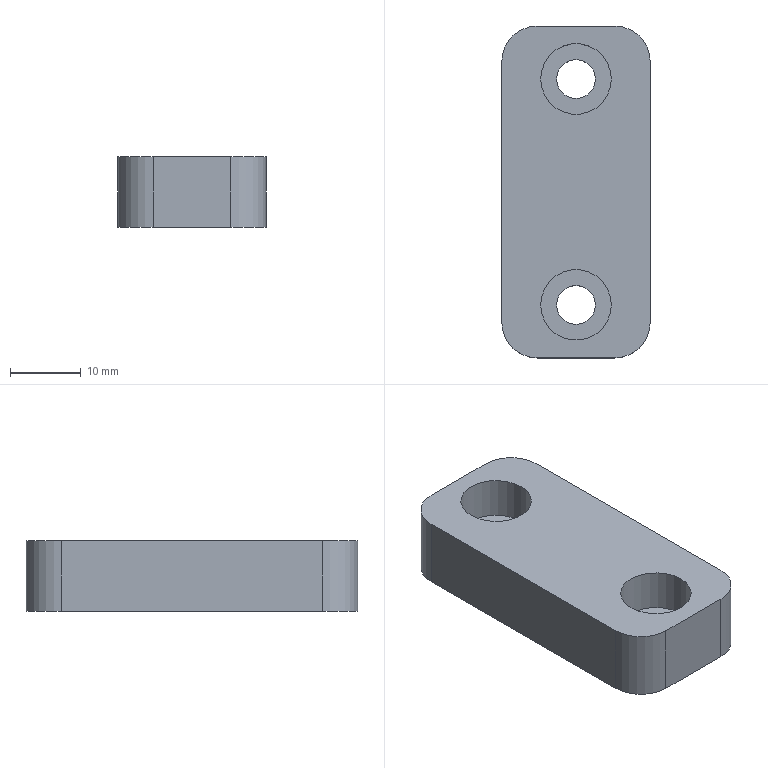Part | STEP file | solid 139 | 1 solid | 16 faces | box 21 x 47 x 10 mm | volume 8523 mm3 | plane 8 | cylinder 8 | commonest cylinder face diameters 10 x6 5.5 x2